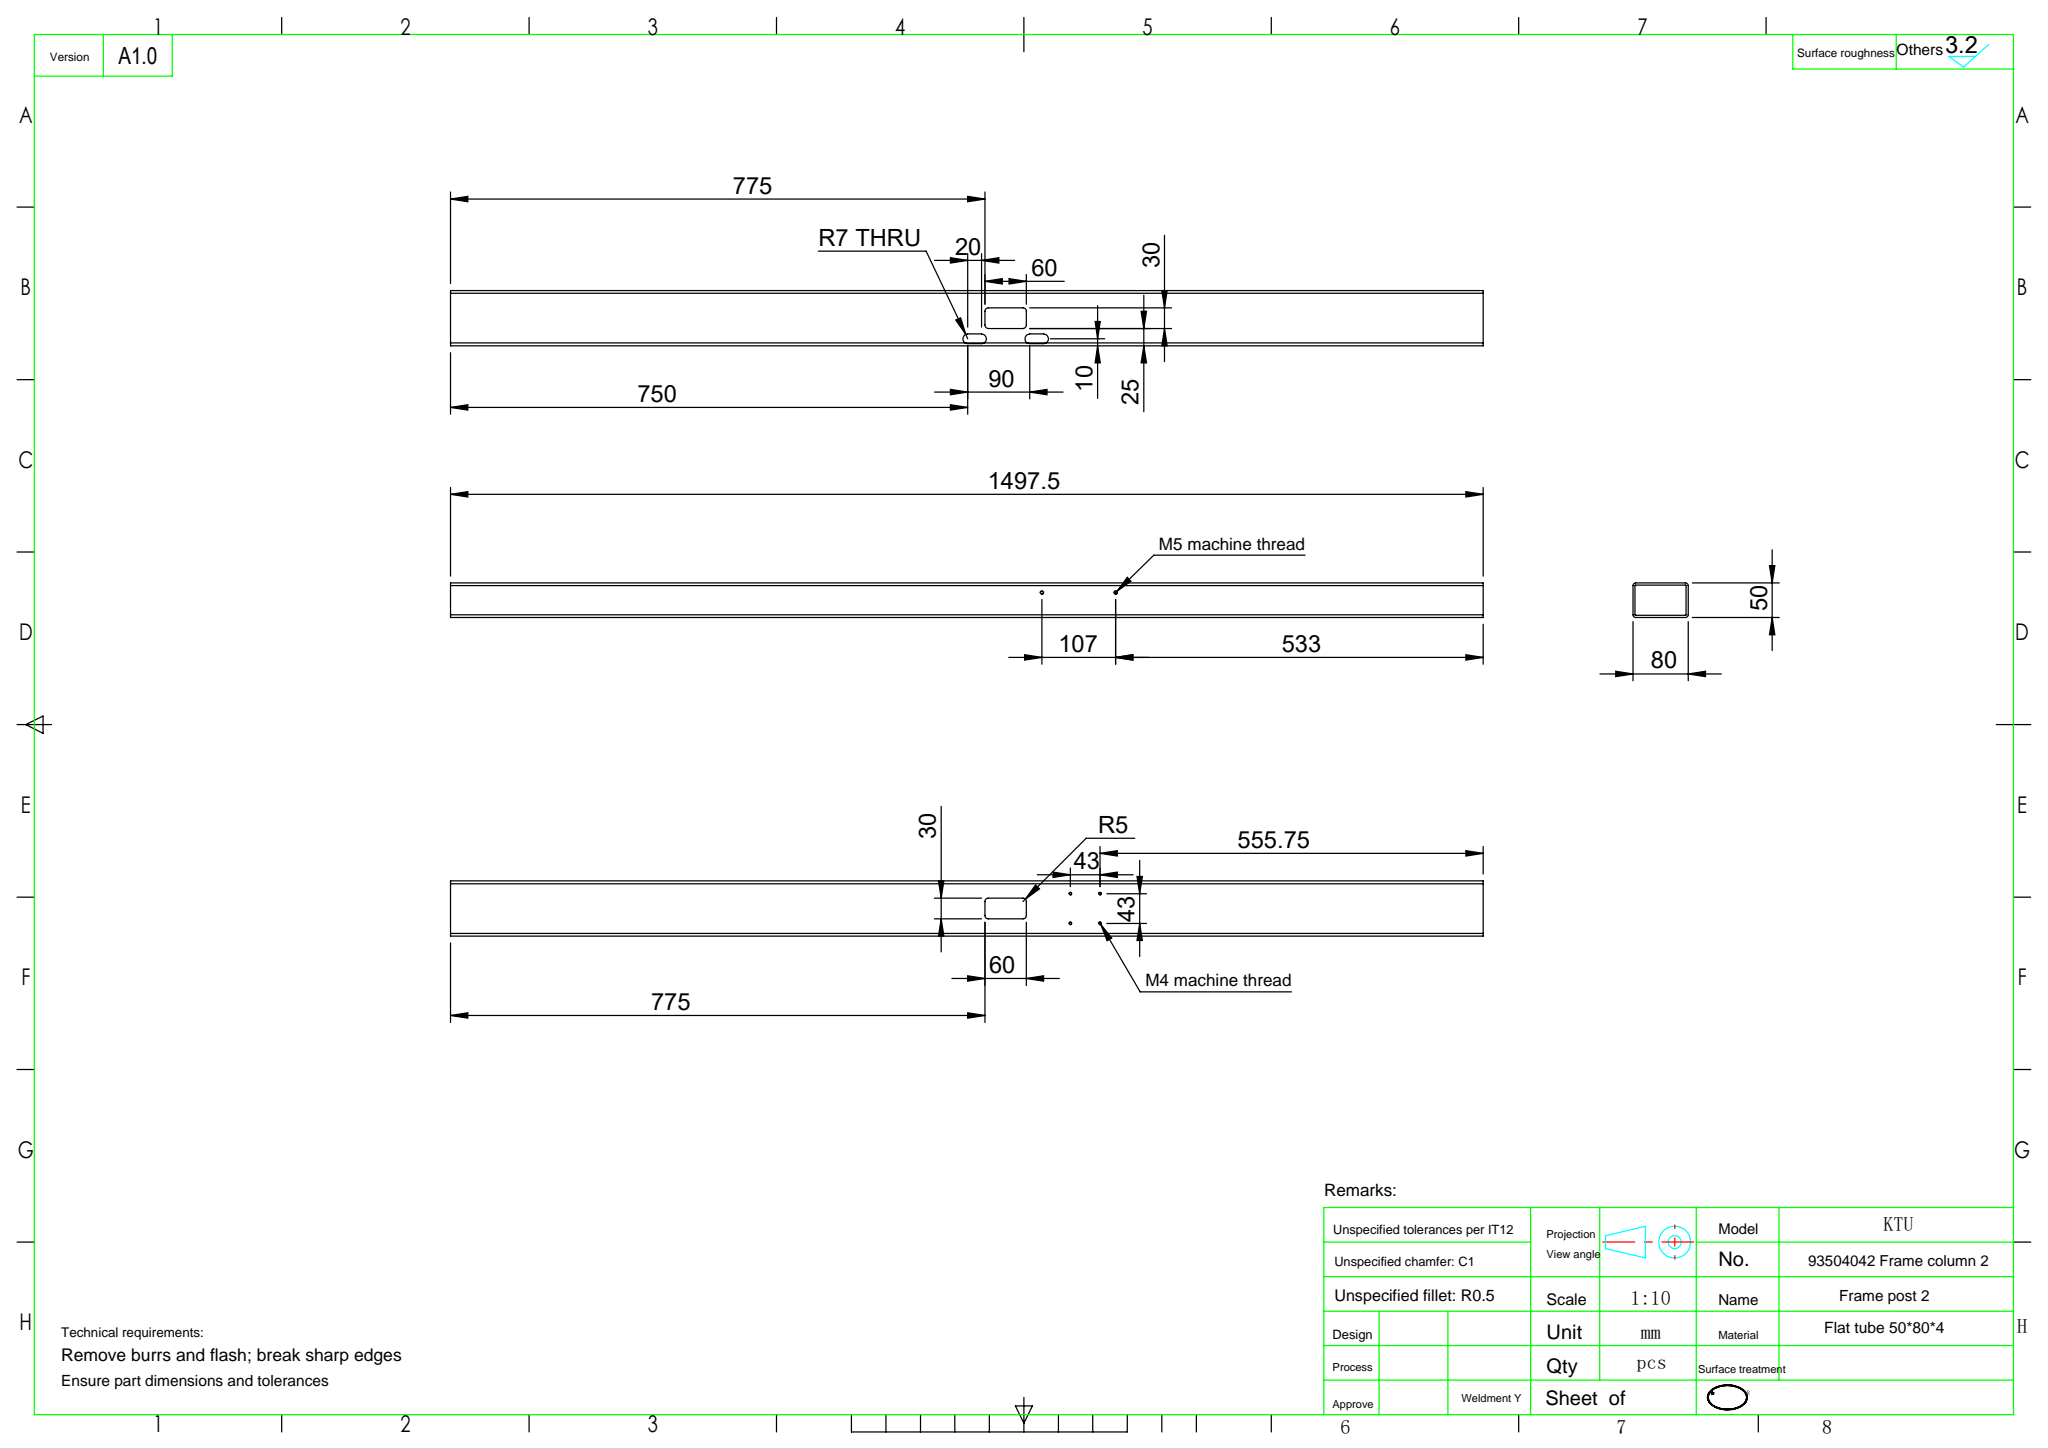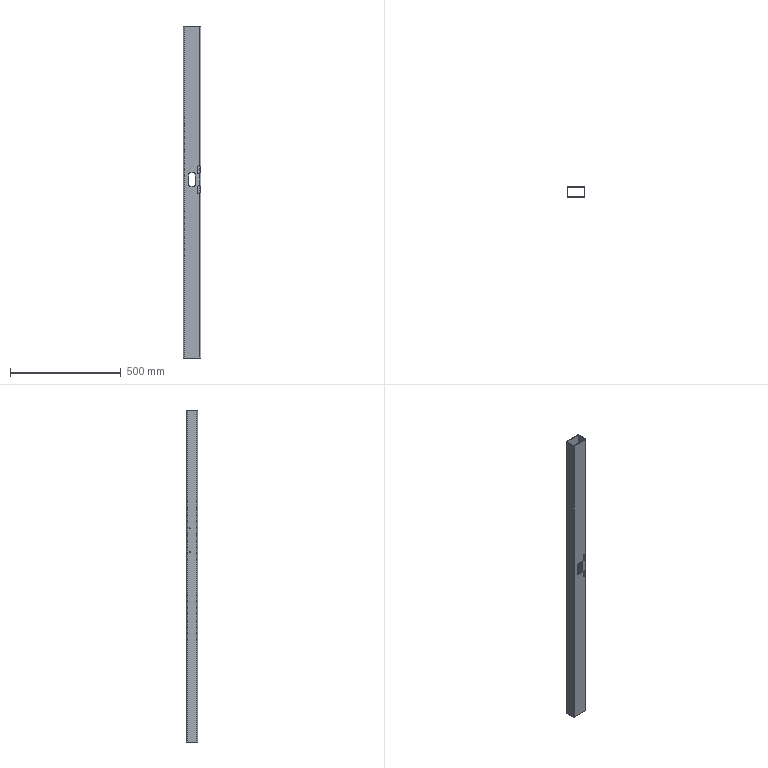Part | SolidWorks | features Cut 2, ICE 2, ExtruThin 1 | 1 solid | 56 faces | box 80 x 50 x 1498 mm | volume 1081389 mm3 | cylinder 36 | plane 20 | commonest cylinder face diameters 3.3 x8 10 x8 2 x6 14 x6 4.2 x4 8 x4